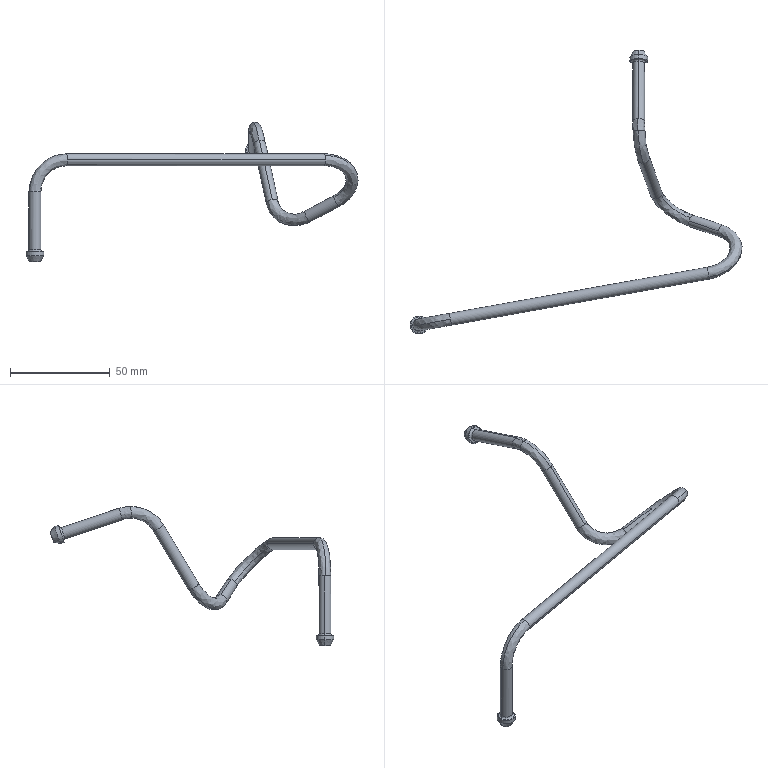Part | SolidWorks | features BaseBody 1 | 1 solid | 68 faces | box 166.262 x 142.113 x 69.761 mm | volume 9860 mm3 | cylinder 28 | spline 24 | cone 12 | plane 4 | commonest cylinder face diameters 1.6 x10 6 x10 2 x4 9 x4